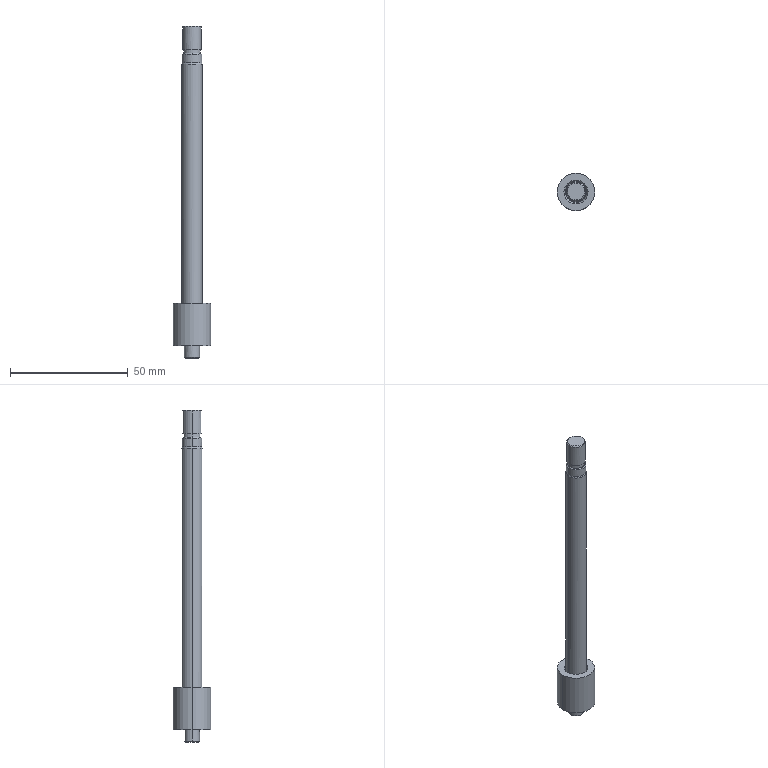Part | SolidWorks | features BaseBody 2, CombineBodies 1, Scale 1 | 1 solid | 50 faces | box 15.92 x 15.92 x 140.8 mm | volume 10674 mm3 | cylinder 22 | cone 17 | plane 11 | commonest cylinder face diameters 8.8 x6 4.8 x2 5.6 x2 6.4 x2 7.04 x2 7.2 x2
STEP:
#1=CARTESIAN_POINT('',(0.,-3.6,68.963));
#2=VERTEX_POINT('',#1);
#3=CARTESIAN_POINT('',(3.6,0.,68.963));
#4=VERTEX_POINT('',#3);
#5=CARTESIAN_POINT('',(0.,0.,68.963));
#6=DIRECTION('',(0.,0.,1.));
#7=DIRECTION('',(-1.,0.,0.));
#8=AXIS2_PLACEMENT_3D('',#5,#6,#7);
#9=CIRCLE('',#8,3.6);
#10=EDGE_CURVE('',#2,#4,#9,.T.);
#11=ORIENTED_EDGE('',*,*,#10,.F.);
#12=CARTESIAN_POINT('',(0.,-4.,68.563));
#13=VERTEX_POINT('',#12);
#14=CARTESIAN_POINT('',(0.,-3.8,68.763));
#15=DIRECTION('',(0.,-0.7071,-0.7071));
#16=VECTOR('',#15,1000.);
#17=LINE('',#14,#16);
#18=EDGE_CURVE('',#2,#13,#17,.T.);
#19=ORIENTED_EDGE('',*,*,#18,.T.);
#20=CARTESIAN_POINT('',(4.,0.,68.563));
#21=VERTEX_POINT('',#20);
#22=CARTESIAN_POINT('',(0.,0.,68.563));
#23=DIRECTION('',(0.,0.,1.));
#24=DIRECTION('',(-1.,0.,0.));
#25=AXIS2_PLACEMENT_3D('',#22,#23,#24);
#26=CIRCLE('',#25,4.);
#27=EDGE_CURVE('',#13,#21,#26,.T.);
#28=ORIENTED_EDGE('',*,*,#27,.T.);
#29=CARTESIAN_POINT('',(3.6,0.000000096,68.963));
#30=DIRECTION('',(0.7071,-0.000000028,-0.7071));
#31=VECTOR('',#30,1000.);
#32=LINE('',#29,#31);
#33=EDGE_CURVE('',#4,#21,#32,.T.);
#34=ORIENTED_EDGE('',*,*,#33,.F.);
#35=EDGE_LOOP('',(#11,#19,#28,#34));
#36=FACE_OUTER_BOUND('',#35,.T.);
#37=CARTESIAN_POINT('',(0.,0.,68.763));
#38=DIRECTION('',(0.,0.,-1.));
#39=DIRECTION('',(0.,-1.,0.));
#40=AXIS2_PLACEMENT_3D('',#37,#38,#39);
#41=CONICAL_SURFACE('',#40,3.8,0.7854);
#42=ADVANCED_FACE('',(#36),#41,.T.);
#43=CARTESIAN_POINT('',(0.,-3.8,57.363));
#44=VERTEX_POINT('',#43);
#45=CARTESIAN_POINT('',(3.8,0.,57.363));
#46=VERTEX_POINT('',#45);
#47=CARTESIAN_POINT('',(0.,0.,57.363));
#48=DIRECTION('',(0.,0.,1.));
#49=DIRECTION('',(-1.,0.,0.));
#50=AXIS2_PLACEMENT_3D('',#47,#48,#49);
#51=CIRCLE('',#50,3.8);
#52=EDGE_CURVE('',#44,#46,#51,.T.);
#53=ORIENTED_EDGE('',*,*,#52,.F.);
#54=CARTESIAN_POINT('',(0.,-4.2,56.963));
#55=VERTEX_POINT('',#54);
#56=CARTESIAN_POINT('',(0.,-4.,57.163));
#57=DIRECTION('',(0.,-0.7071,-0.7071));
#58=VECTOR('',#57,1000.);
#59=LINE('',#56,#58);
#60=EDGE_CURVE('',#44,#55,#59,.T.);
#61=ORIENTED_EDGE('',*,*,#60,.T.);
#62=CARTESIAN_POINT('',(4.2,0.,56.963));
#63=VERTEX_POINT('',#62);
#64=CARTESIAN_POINT('',(0.,0.,56.963));
#65=DIRECTION('',(0.,0.,1.));
#66=DIRECTION('',(-1.,0.,0.));
#67=AXIS2_PLACEMENT_3D('',#64,#65,#66);
#68=CIRCLE('',#67,4.2);
#69=EDGE_CURVE('',#55,#63,#68,.T.);
#70=ORIENTED_EDGE('',*,*,#69,.T.);
#71=CARTESIAN_POINT('',(3.8,0.000000099,57.363));
#72=DIRECTION('',(0.7071,-0.00000003,-0.7071));
#73=VECTOR('',#72,1000.);
#74=LINE('',#71,#73);
#75=EDGE_CURVE('',#46,#63,#74,.T.);
#76=ORIENTED_EDGE('',*,*,#75,.F.);
#77=EDGE_LOOP('',(#53,#61,#70,#76));
#78=FACE_OUTER_BOUND('',#77,.T.);
#79=CARTESIAN_POINT('',(0.,0.,57.163));
#80=DIRECTION('',(0.,0.,-1.));
#81=DIRECTION('',(0.,-1.,0.));
#82=AXIS2_PLACEMENT_3D('',#79,#80,#81);
#83=CONICAL_SURFACE('',#82,4.,0.7854);
#84=ADVANCED_FACE('',(#78),#83,.T.);
#85=CARTESIAN_POINT('',(-2.8,0.,-71.837));
#86=VERTEX_POINT('',#85);
#87=CARTESIAN_POINT('',(0.,-2.8,-71.837));
#88=VERTEX_POINT('',#87);
#89=CARTESIAN_POINT('',(0.,0.,-71.837));
#90=DIRECTION('',(0.,0.,1.));
#91=DIRECTION('',(-1.,0.,0.));
#92=AXIS2_PLACEMENT_3D('',#89,#90,#91);
#93=CIRCLE('',#92,2.8);
#94=EDGE_CURVE('',#86,#88,#93,.T.);
#95=ORIENTED_EDGE('',*,*,#94,.T.);
#96=CARTESIAN_POINT('',(0.,-3.2,-71.437));
#97=VERTEX_POINT('',#96);
#98=CARTESIAN_POINT('',(0.,-3.,-71.637));
#99=DIRECTION('',(0.,-0.7071,0.7071));
#100=VECTOR('',#99,1000.);
#101=LINE('',#98,#100);
#102=EDGE_CURVE('',#88,#97,#101,.T.);
#103=ORIENTED_EDGE('',*,*,#102,.T.);
#104=CARTESIAN_POINT('',(-3.2,0.,-71.437));
#105=VERTEX_POINT('',#104);
#106=CARTESIAN_POINT('',(0.,0.,-71.437));
#107=DIRECTION('',(0.,0.,1.));
#108=DIRECTION('',(-1.,0.,0.));
#109=AXIS2_PLACEMENT_3D('',#106,#107,#108);
#110=CIRCLE('',#109,3.2);
#111=EDGE_CURVE('',#105,#97,#110,.T.);
#112=ORIENTED_EDGE('',*,*,#111,.F.);
#113=CARTESIAN_POINT('',(-3.2,0.000000012,-71.437));
#114=DIRECTION('',(0.7071,0.000000004,-0.7071));
#115=VECTOR('',#114,1000.);
#116=LINE('',#113,#115);
#117=EDGE_CURVE('',#105,#86,#116,.T.);
#118=ORIENTED_EDGE('',*,*,#117,.T.);
#119=EDGE_LOOP('',(#95,#103,#112,#118));
#120=FACE_OUTER_BOUND('',#119,.T.);
#121=CARTESIAN_POINT('',(0.,0.,-71.637));
#122=DIRECTION('',(0.,0.,1.));
#123=DIRECTION('',(0.,-1.,0.));
#124=AXIS2_PLACEMENT_3D('',#121,#122,#123);
#125=CONICAL_SURFACE('',#124,3.,0.7854);
#126=ADVANCED_FACE('',(#120),#125,.T.);
#127=CARTESIAN_POINT('',(0.,-4.4,-49.837));
#128=VERTEX_POINT('',#127);
#129=CARTESIAN_POINT('',(4.4,0.,-49.837));
#130=VERTEX_POINT('',#129);
#131=CARTESIAN_POINT('',(0.,0.,-49.837));
#132=DIRECTION('',(0.,0.,1.));
#133=DIRECTION('',(-1.,0.,0.));
#134=AXIS2_PLACEMENT_3D('',#131,#132,#133);
#135=CIRCLE('',#134,4.4);
#136=EDGE_CURVE('',#128,#130,#135,.T.);
#137=ORIENTED_EDGE('',*,*,#136,.F.);
#138=CARTESIAN_POINT('',(0.,-5.093,-48.637));
#139=VERTEX_POINT('',#138);
#140=CARTESIAN_POINT('',(0.,-4.746,-49.237));
#141=DIRECTION('',(0.,-0.5,0.866));
#142=VECTOR('',#141,1000.);
#143=LINE('',#140,#142);
#144=EDGE_CURVE('',#128,#139,#143,.T.);
#145=ORIENTED_EDGE('',*,*,#144,.T.);
#146=CARTESIAN_POINT('',(5.093,0.,-48.637));
#147=VERTEX_POINT('',#146);
#148=CARTESIAN_POINT('',(0.,0.,-48.637));
#149=DIRECTION('',(0.,0.,1.));
#150=DIRECTION('',(-1.,0.,0.));
#151=AXIS2_PLACEMENT_3D('',#148,#149,#150);
#152=CIRCLE('',#151,5.093);
#153=EDGE_CURVE('',#139,#147,#152,.T.);
#154=ORIENTED_EDGE('',*,*,#153,.T.);
#155=CARTESIAN_POINT('',(4.4,0.000000001,-49.837));
#156=DIRECTION('',(0.5,0.,0.866));
#157=VECTOR('',#156,1000.);
#158=LINE('',#155,#157);
#159=EDGE_CURVE('',#130,#147,#158,.T.);
#160=ORIENTED_EDGE('',*,*,#159,.F.);
#161=EDGE_LOOP('',(#137,#145,#154,#160));
#162=FACE_OUTER_BOUND('',#161,.T.);
#163=CARTESIAN_POINT('',(0.,0.,-49.237));
#164=DIRECTION('',(0.,0.,1.));
#165=DIRECTION('',(0.,-1.,0.));
#166=AXIS2_PLACEMENT_3D('',#163,#164,#165);
#167=CONICAL_SURFACE('',#166,4.746,0.5236);
#168=ADVANCED_FACE('',(#162),#167,.F.);
#169=CARTESIAN_POINT('',(-7.96,0.,-48.637));
#170=VERTEX_POINT('',#169);
#171=CARTESIAN_POINT('',(7.96,0.,-48.637));
#172=VERTEX_POINT('',#171);
#173=CARTESIAN_POINT('',(0.,0.,-48.637));
#174=DIRECTION('',(0.,0.,-1.));
#175=DIRECTION('',(-1.,0.,0.));
#176=AXIS2_PLACEMENT_3D('',#173,#174,#175);
#177=CIRCLE('',#176,7.96);
#178=EDGE_CURVE('',#170,#172,#177,.T.);
#179=ORIENTED_EDGE('',*,*,#178,.F.);
#180=CARTESIAN_POINT('',(0.,0.,-48.637));
#181=DIRECTION('',(0.,0.,1.));
#182=DIRECTION('',(-1.,0.,0.));
#183=AXIS2_PLACEMENT_3D('',#180,#181,#182);
#184=CIRCLE('',#183,7.96);
#185=EDGE_CURVE('',#170,#172,#184,.T.);
#186=ORIENTED_EDGE('',*,*,#185,.T.);
#187=EDGE_LOOP('',(#179,#186));
#188=FACE_OUTER_BOUND('',#187,.T.);
#189=CARTESIAN_POINT('',(-5.093,0.,-48.637));
#190=VERTEX_POINT('',#189);
#191=CARTESIAN_POINT('',(0.,0.,-48.637));
#192=DIRECTION('',(0.,0.,1.));
#193=DIRECTION('',(1.,0.,0.));
#194=AXIS2_PLACEMENT_3D('',#191,#192,#193);
#195=CIRCLE('',#194,5.093);
#196=EDGE_CURVE('',#147,#190,#195,.T.);
#197=ORIENTED_EDGE('',*,*,#196,.F.);
#198=ORIENTED_EDGE('',*,*,#153,.F.);
#199=CARTESIAN_POINT('',(0.,0.,-48.637));
#200=DIRECTION('',(0.,0.,1.));
#201=DIRECTION('',(-1.,0.,0.));
#202=AXIS2_PLACEMENT_3D('',#199,#200,#201);
#203=CIRCLE('',#202,5.093);
#204=EDGE_CURVE('',#190,#139,#203,.T.);
#205=ORIENTED_EDGE('',*,*,#204,.F.);
#206=EDGE_LOOP('',(#197,#198,#205));
#207=FACE_BOUND('',#206,.T.);
#208=CARTESIAN_POINT('',(0.,0.,-48.637));
#209=DIRECTION('',(0.,0.,-1.));
#210=DIRECTION('',(0.,-1.,0.));
#211=AXIS2_PLACEMENT_3D('',#208,#209,#210);
#212=PLANE('',#211);
#213=ADVANCED_FACE('',(#188,#207),#212,.F.);
#214=CARTESIAN_POINT('',(-7.96,0.,-66.637));
#215=VERTEX_POINT('',#214);
#216=CARTESIAN_POINT('',(7.96,0.,-66.637));
#217=VERTEX_POINT('',#216);
#218=CARTESIAN_POINT('',(0.,0.,-66.637));
#219=DIRECTION('',(0.,0.,1.));
#220=DIRECTION('',(-1.,0.,0.));
#221=AXIS2_PLACEMENT_3D('',#218,#219,#220);
#222=CIRCLE('',#221,7.96);
#223=EDGE_CURVE('',#215,#217,#222,.T.);
#224=ORIENTED_EDGE('',*,*,#223,.T.);
#225=CARTESIAN_POINT('',(7.96,0.,-66.637));
#226=DIRECTION('',(0.,0.,1.));
#227=VECTOR('',#226,1000.);
#228=LINE('',#225,#227);
#229=EDGE_CURVE('',#217,#172,#228,.T.);
#230=ORIENTED_EDGE('',*,*,#229,.T.);
#231=ORIENTED_EDGE('',*,*,#185,.F.);
#232=CARTESIAN_POINT('',(-7.96,0.,-66.637));
#233=DIRECTION('',(0.,0.,1.));
#234=VECTOR('',#233,1000.);
#235=LINE('',#232,#234);
#236=EDGE_CURVE('',#215,#170,#235,.T.);
#237=ORIENTED_EDGE('',*,*,#236,.F.);
#238=EDGE_LOOP('',(#224,#230,#231,#237));
#239=FACE_OUTER_BOUND('',#238,.T.);
#240=CARTESIAN_POINT('',(0.,0.,-47.737));
#241=DIRECTION('',(0.,0.,-1.));
#242=DIRECTION('',(1.,0.,0.));
#243=AXIS2_PLACEMENT_3D('',#240,#241,#242);
#244=CYLINDRICAL_SURFACE('',#243,7.96);
#245=ADVANCED_FACE('',(#239),#244,.T.);
#246=ORIENTED_EDGE('',*,*,#178,.T.);
#247=ORIENTED_EDGE('',*,*,#229,.F.);
#248=CARTESIAN_POINT('',(0.,0.,-66.637));
#249=DIRECTION('',(0.,0.,-1.));
#250=DIRECTION('',(-1.,0.,0.));
#251=AXIS2_PLACEMENT_3D('',#248,#249,#250);
#252=CIRCLE('',#251,7.96);
#253=EDGE_CURVE('',#215,#217,#252,.T.);
#254=ORIENTED_EDGE('',*,*,#253,.F.);
#255=ORIENTED_EDGE('',*,*,#236,.T.);
#256=EDGE_LOOP('',(#246,#247,#254,#255));
#257=FACE_OUTER_BOUND('',#256,.T.);
#258=CARTESIAN_POINT('',(0.,0.,-47.737));
#259=DIRECTION('',(0.,0.,-1.));
#260=DIRECTION('',(1.,0.,0.));
#261=AXIS2_PLACEMENT_3D('',#258,#259,#260);
#262=CYLINDRICAL_SURFACE('',#261,7.96);
#263=ADVANCED_FACE('',(#257),#262,.T.);
#264=CARTESIAN_POINT('',(3.2,-0.000000008,-66.637));
#265=VERTEX_POINT('',#264);
#266=CARTESIAN_POINT('',(-3.2,0.,-66.637));
#267=VERTEX_POINT('',#266);
#268=CARTESIAN_POINT('',(0.,0.,-66.637));
#269=DIRECTION('',(0.,0.,-1.));
#270=DIRECTION('',(-1.,0.,0.));
#271=AXIS2_PLACEMENT_3D('',#268,#269,#270);
#272=CIRCLE('',#271,3.2);
#273=EDGE_CURVE('',#265,#267,#272,.T.);
#274=ORIENTED_EDGE('',*,*,#273,.F.);
#275=CARTESIAN_POINT('',(0.,0.,-66.637));
#276=DIRECTION('',(0.,0.,-1.));
#277=DIRECTION('',(-1.,0.,0.));
#278=AXIS2_PLACEMENT_3D('',#275,#276,#277);
#279=CIRCLE('',#278,3.2);
#280=EDGE_CURVE('',#267,#265,#279,.T.);
#281=ORIENTED_EDGE('',*,*,#280,.F.);
#282=EDGE_LOOP('',(#274,#281));
#283=FACE_BOUND('',#282,.T.);
#284=ORIENTED_EDGE('',*,*,#223,.F.);
#285=ORIENTED_EDGE('',*,*,#253,.T.);
#286=EDGE_LOOP('',(#284,#285));
#287=FACE_OUTER_BOUND('',#286,.T.);
#288=CARTESIAN_POINT('',(0.,0.,-66.637));
#289=DIRECTION('',(0.,0.,-1.));
#290=DIRECTION('',(0.,-1.,0.));
#291=AXIS2_PLACEMENT_3D('',#288,#289,#290);
#292=PLANE('',#291);
#293=ADVANCED_FACE('',(#283,#287),#292,.T.);
#294=ORIENTED_EDGE('',*,*,#144,.F.);
#295=CARTESIAN_POINT('',(-4.4,0.,-49.837));
#296=VERTEX_POINT('',#295);
#297=CARTESIAN_POINT('',(0.,0.,-49.837));
#298=DIRECTION('',(0.,0.,1.));
#299=DIRECTION('',(-1.,0.,0.));
#300=AXIS2_PLACEMENT_3D('',#297,#298,#299);
#301=CIRCLE('',#300,4.4);
#302=EDGE_CURVE('',#296,#128,#301,.T.);
#303=ORIENTED_EDGE('',*,*,#302,.F.);
#304=CARTESIAN_POINT('',(-4.4,-0.000000001,-49.837));
#305=DIRECTION('',(-0.5,0.,0.866));
#306=VECTOR('',#305,1000.);
#307=LINE('',#304,#306);
#308=EDGE_CURVE('',#296,#190,#307,.T.);
#309=ORIENTED_EDGE('',*,*,#308,.T.);
#310=ORIENTED_EDGE('',*,*,#204,.T.);
#311=EDGE_LOOP('',(#294,#303,#309,#310));
#312=FACE_OUTER_BOUND('',#311,.T.);
#313=CARTESIAN_POINT('',(0.,0.,-49.237));
#314=DIRECTION('',(0.,0.,1.));
#315=DIRECTION('',(0.,-1.,0.));
#316=AXIS2_PLACEMENT_3D('',#313,#314,#315);
#317=CONICAL_SURFACE('',#316,4.746,0.5236);
#318=ADVANCED_FACE('',(#312),#317,.F.);
#319=ORIENTED_EDGE('',*,*,#159,.T.);
#320=ORIENTED_EDGE('',*,*,#196,.T.);
#321=ORIENTED_EDGE('',*,*,#308,.F.);
#322=CARTESIAN_POINT('',(0.,0.,-49.837));
#323=DIRECTION('',(0.,0.,1.));
#324=DIRECTION('',(1.,0.,0.));
#325=AXIS2_PLACEMENT_3D('',#322,#323,#324);
#326=CIRCLE('',#325,4.4);
#327=EDGE_CURVE('',#130,#296,#326,.T.);
#328=ORIENTED_EDGE('',*,*,#327,.F.);
#329=EDGE_LOOP('',(#319,#320,#321,#328));
#330=FACE_OUTER_BOUND('',#329,.T.);
#331=CARTESIAN_POINT('',(0.,0.,-49.237));
#332=DIRECTION('',(0.,0.,1.));
#333=DIRECTION('',(0.,-1.,0.));
#334=AXIS2_PLACEMENT_3D('',#331,#332,#333);
#335=CONICAL_SURFACE('',#334,4.746,0.5236);
#336=ADVANCED_FACE('',(#330),#335,.F.);
#337=CARTESIAN_POINT('',(2.8,0.,-71.837));
#338=VERTEX_POINT('',#337);
#339=CARTESIAN_POINT('',(0.,0.,-71.837));
#340=DIRECTION('',(0.,0.,1.));
#341=DIRECTION('',(1.,0.,0.));
#342=AXIS2_PLACEMENT_3D('',#339,#340,#341);
#343=CIRCLE('',#342,2.8);
#344=EDGE_CURVE('',#338,#86,#343,.T.);
#345=ORIENTED_EDGE('',*,*,#344,.F.);
#346=CARTESIAN_POINT('',(0.,0.,-71.837));
#347=DIRECTION('',(0.,0.,1.));
#348=DIRECTION('',(-1.,0.,0.));
#349=AXIS2_PLACEMENT_3D('',#346,#347,#348);
#350=CIRCLE('',#349,2.8);
#351=EDGE_CURVE('',#88,#338,#350,.T.);
#352=ORIENTED_EDGE('',*,*,#351,.F.);
#353=ORIENTED_EDGE('',*,*,#94,.F.);
#354=EDGE_LOOP('',(#345,#352,#353));
#355=FACE_OUTER_BOUND('',#354,.T.);
#356=CARTESIAN_POINT('',(0.,0.,-71.837));
#357=DIRECTION('',(0.,0.,-1.));
#358=DIRECTION('',(0.,-1.,0.));
#359=AXIS2_PLACEMENT_3D('',#356,#357,#358);
#360=PLANE('',#359);
#361=ADVANCED_FACE('',(#355),#360,.T.);
#362=ORIENTED_EDGE('',*,*,#102,.F.);
#363=ORIENTED_EDGE('',*,*,#351,.T.);
#364=CARTESIAN_POINT('',(3.2,0.,-71.437));
#365=VERTEX_POINT('',#364);
#366=CARTESIAN_POINT('',(3.2,-0.000000012,-71.437));
#367=DIRECTION('',(-0.7071,-0.000000004,-0.7071));
#368=VECTOR('',#367,1000.);
#369=LINE('',#366,#368);
#370=EDGE_CURVE('',#365,#338,#369,.T.);
#371=ORIENTED_EDGE('',*,*,#370,.F.);
#372=CARTESIAN_POINT('',(0.,0.,-71.437));
#373=DIRECTION('',(0.,0.,1.));
#374=DIRECTION('',(-1.,0.,0.));
#375=AXIS2_PLACEMENT_3D('',#372,#373,#374);
#376=CIRCLE('',#375,3.2);
#377=EDGE_CURVE('',#97,#365,#376,.T.);
#378=ORIENTED_EDGE('',*,*,#377,.F.);
#379=EDGE_LOOP('',(#362,#363,#371,#378));
#380=FACE_OUTER_BOUND('',#379,.T.);
#381=CARTESIAN_POINT('',(0.,0.,-71.637));
#382=DIRECTION('',(0.,0.,1.));
#383=DIRECTION('',(0.,-1.,0.));
#384=AXIS2_PLACEMENT_3D('',#381,#382,#383);
#385=CONICAL_SURFACE('',#384,3.,0.7854);
#386=ADVANCED_FACE('',(#380),#385,.T.);
#387=ORIENTED_EDGE('',*,*,#370,.T.);
#388=ORIENTED_EDGE('',*,*,#344,.T.);
#389=ORIENTED_EDGE('',*,*,#117,.F.);
#390=CARTESIAN_POINT('',(0.,0.,-71.437));
#391=DIRECTION('',(0.,0.,1.));
#392=DIRECTION('',(1.,0.,0.));
#393=AXIS2_PLACEMENT_3D('',#390,#391,#392);
#394=CIRCLE('',#393,3.2);
#395=EDGE_CURVE('',#365,#105,#394,.T.);
#396=ORIENTED_EDGE('',*,*,#395,.F.);
#397=EDGE_LOOP('',(#387,#388,#389,#396));
#398=FACE_OUTER_BOUND('',#397,.T.);
#399=CARTESIAN_POINT('',(0.,0.,-71.637));
#400=DIRECTION('',(0.,0.,1.));
#401=DIRECTION('',(0.,-1.,0.));
#402=AXIS2_PLACEMENT_3D('',#399,#400,#401);
#403=CONICAL_SURFACE('',#402,3.,0.7854);
#404=ADVANCED_FACE('',(#398),#403,.T.);
#405=CARTESIAN_POINT('',(-3.2,0.000000012,-71.437));
#406=DIRECTION('',(-0.000000001,-0.000000001,1.));
#407=VECTOR('',#406,1000.);
#408=LINE('',#405,#407);
#409=EDGE_CURVE('',#105,#267,#408,.T.);
#410=ORIENTED_EDGE('',*,*,#409,.T.);
#411=ORIENTED_EDGE('',*,*,#280,.T.);
#412=CARTESIAN_POINT('',(3.2,-0.000000012,-71.437));
#413=DIRECTION('',(0.000000001,0.000000001,1.));
#414=VECTOR('',#413,1000.);
#415=LINE('',#412,#414);
#416=EDGE_CURVE('',#365,#265,#415,.T.);
#417=ORIENTED_EDGE('',*,*,#416,.F.);
#418=ORIENTED_EDGE('',*,*,#395,.T.);
#419=EDGE_LOOP('',(#410,#411,#417,#418));
#420=FACE_OUTER_BOUND('',#419,.T.);
#421=CARTESIAN_POINT('',(0.,0.,76.239));
#422=DIRECTION('',(0.,0.,-1.));
#423=DIRECTION('',(1.,0.,0.));
#424=AXIS2_PLACEMENT_3D('',#421,#422,#423);
#425=CYLINDRICAL_SURFACE('',#424,3.2);
#426=ADVANCED_FACE('',(#420),#425,.T.);
#427=ORIENTED_EDGE('',*,*,#416,.T.);
#428=ORIENTED_EDGE('',*,*,#273,.T.);
#429=ORIENTED_EDGE('',*,*,#409,.F.);
#430=ORIENTED_EDGE('',*,*,#111,.T.);
#431=ORIENTED_EDGE('',*,*,#377,.T.);
#432=EDGE_LOOP('',(#427,#428,#429,#430,#431));
#433=FACE_OUTER_BOUND('',#432,.T.);
#434=CARTESIAN_POINT('',(0.,0.,76.239));
#435=DIRECTION('',(0.,0.,-1.));
#436=DIRECTION('',(1.,0.,0.));
#437=AXIS2_PLACEMENT_3D('',#434,#435,#436);
#438=CYLINDRICAL_SURFACE('',#437,3.2);
#439=ADVANCED_FACE('',(#433),#438,.T.);
#440=CARTESIAN_POINT('',(-4.4,0.,52.813));
#441=VERTEX_POINT('',#440);
#442=CARTESIAN_POINT('',(-4.4,0.,-51.197));
#443=DIRECTION('',(0.,0.,1.));
#444=VECTOR('',#443,1000.);
#445=LINE('',#442,#444);
#446=EDGE_CURVE('',#296,#441,#445,.T.);
#447=ORIENTED_EDGE('',*,*,#446,.F.);
#448=ORIENTED_EDGE('',*,*,#302,.T.);
#449=ORIENTED_EDGE('',*,*,#136,.T.);
#450=CARTESIAN_POINT('',(4.4,0.,52.813));
#451=VERTEX_POINT('',#450);
#452=CARTESIAN_POINT('',(4.4,0.,-51.197));
#453=DIRECTION('',(0.,0.,1.));
#454=VECTOR('',#453,1000.);
#455=LINE('',#452,#454);
#456=EDGE_CURVE('',#130,#451,#455,.T.);
#457=ORIENTED_EDGE('',*,*,#456,.T.);
#458=CARTESIAN_POINT('',(0.,0.,52.813));
#459=DIRECTION('',(0.,0.,1.));
#460=DIRECTION('',(-1.,0.,0.));
#461=AXIS2_PLACEMENT_3D('',#458,#459,#460);
#462=CIRCLE('',#461,4.4);
#463=EDGE_CURVE('',#441,#451,#462,.T.);
#464=ORIENTED_EDGE('',*,*,#463,.F.);
#465=EDGE_LOOP('',(#447,#448,#449,#457,#464));
#466=FACE_OUTER_BOUND('',#465,.T.);
#467=CARTESIAN_POINT('',(0.,0.,76.239));
#468=DIRECTION('',(0.,0.,-1.));
#469=DIRECTION('',(1.,0.,0.));
#470=AXIS2_PLACEMENT_3D('',#467,#468,#469);
#471=CYLINDRICAL_SURFACE('',#470,4.4);
#472=ADVANCED_FACE('',(#466),#471,.T.);
#473=ORIENTED_EDGE('',*,*,#456,.F.);
#474=ORIENTED_EDGE('',*,*,#327,.T.);
#475=ORIENTED_EDGE('',*,*,#446,.T.);
#476=CARTESIAN_POINT('',(0.,0.,52.813));
#477=DIRECTION('',(0.,0.,-1.));
#478=DIRECTION('',(-1.,0.,0.));
#479=AXIS2_PLACEMENT_3D('',#476,#477,#478);
#480=CIRCLE('',#479,4.4);
#481=EDGE_CURVE('',#441,#451,#480,.T.);
#482=ORIENTED_EDGE('',*,*,#481,.T.);
#483=EDGE_LOOP('',(#473,#474,#475,#482));
#484=FACE_OUTER_BOUND('',#483,.T.);
#485=CARTESIAN_POINT('',(0.,0.,76.239));
#486=DIRECTION('',(0.,0.,-1.));
#487=DIRECTION('',(1.,0.,0.));
#488=AXIS2_PLACEMENT_3D('',#485,#486,#487);
#489=CYLINDRICAL_SURFACE('',#488,4.4);
#490=ADVANCED_FACE('',(#484),#489,.T.);
#491=CARTESIAN_POINT('',(-4.2,0.,53.363));
#492=VERTEX_POINT('',#491);
#493=CARTESIAN_POINT('',(4.2,0.,53.363));
#494=VERTEX_POINT('',#493);
#495=CARTESIAN_POINT('',(0.,0.,53.363));
#496=DIRECTION('',(0.,0.,-1.));
#497=DIRECTION('',(-1.,0.,0.));
#498=AXIS2_PLACEMENT_3D('',#495,#496,#497);
#499=CIRCLE('',#498,4.2);
#500=EDGE_CURVE('',#492,#494,#499,.T.);
#501=ORIENTED_EDGE('',*,*,#500,.T.);
#502=CARTESIAN_POINT('',(4.4,0.,52.813));
#503=DIRECTION('',(-0.342,0.,0.9397));
#504=VECTOR('',#503,1000.);
#505=LINE('',#502,#504);
#506=EDGE_CURVE('',#451,#494,#505,.T.);
#507=ORIENTED_EDGE('',*,*,#506,.F.);
#508=ORIENTED_EDGE('',*,*,#481,.F.);
#509=CARTESIAN_POINT('',(-4.4,0.,52.813));
#510=DIRECTION('',(0.342,0.,0.9397));
#511=VECTOR('',#510,1000.);
#512=LINE('',#509,#511);
#513=EDGE_CURVE('',#441,#492,#512,.T.);
#514=ORIENTED_EDGE('',*,*,#513,.T.);
#515=EDGE_LOOP('',(#501,#507,#508,#514));
#516=FACE_OUTER_BOUND('',#515,.T.);
#517=CARTESIAN_POINT('',(0.,0.,53.088));
#518=DIRECTION('',(0.,0.,-1.));
#519=DIRECTION('',(1.,0.,0.));
#520=AXIS2_PLACEMENT_3D('',#517,#518,#519);
#521=CONICAL_SURFACE('',#520,4.3,0.3491);
#522=ADVANCED_FACE('',(#516),#521,.T.);
#523=ORIENTED_EDGE('',*,*,#463,.T.);
#524=ORIENTED_EDGE('',*,*,#506,.T.);
#525=CARTESIAN_POINT('',(0.,0.,53.363));
#526=DIRECTION('',(0.,0.,1.));
#527=DIRECTION('',(-1.,0.,0.));
#528=AXIS2_PLACEMENT_3D('',#525,#526,#527);
#529=CIRCLE('',#528,4.2);
#530=EDGE_CURVE('',#492,#494,#529,.T.);
#531=ORIENTED_EDGE('',*,*,#530,.F.);
#532=ORIENTED_EDGE('',*,*,#513,.F.);
#533=EDGE_LOOP('',(#523,#524,#531,#532));
#534=FACE_OUTER_BOUND('',#533,.T.);
#535=CARTESIAN_POINT('',(0.,0.,53.088));
#536=DIRECTION('',(0.,0.,-1.));
#537=DIRECTION('',(1.,0.,0.));
#538=AXIS2_PLACEMENT_3D('',#535,#536,#537);
#539=CONICAL_SURFACE('',#538,4.3,0.3491);
#540=ADVANCED_FACE('',(#534),#539,.T.);
#541=CARTESIAN_POINT('',(-4.2,0.,56.963));
#542=VERTEX_POINT('',#541);
#543=CARTESIAN_POINT('',(-4.2,0.,53.363));
#544=DIRECTION('',(0.000000004,-0.000000023,1.));
#545=VECTOR('',#544,1000.);
#546=LINE('',#543,#545);
#547=EDGE_CURVE('',#492,#542,#546,.T.);
#548=ORIENTED_EDGE('',*,*,#547,.F.);
#549=ORIENTED_EDGE('',*,*,#530,.T.);
#550=CARTESIAN_POINT('',(4.2,0.,53.363));
#551=DIRECTION('',(-0.000000004,0.000000023,1.));
#552=VECTOR('',#551,1000.);
#553=LINE('',#550,#552);
#554=EDGE_CURVE('',#494,#63,#553,.T.);
#555=ORIENTED_EDGE('',*,*,#554,.T.);
#556=ORIENTED_EDGE('',*,*,#69,.F.);
#557=CARTESIAN_POINT('',(0.,0.,56.963));
#558=DIRECTION('',(0.,0.,1.));
#559=DIRECTION('',(-1.,0.,0.));
#560=AXIS2_PLACEMENT_3D('',#557,#558,#559);
#561=CIRCLE('',#560,4.2);
#562=EDGE_CURVE('',#542,#55,#561,.T.);
#563=ORIENTED_EDGE('',*,*,#562,.F.);
#564=EDGE_LOOP('',(#548,#549,#555,#556,#563));
#565=FACE_OUTER_BOUND('',#564,.T.);
#566=CARTESIAN_POINT('',(0.,0.,76.239));
#567=DIRECTION('',(0.,0.,-1.));
#568=DIRECTION('',(1.,0.,0.));
#569=AXIS2_PLACEMENT_3D('',#566,#567,#568);
#570=CYLINDRICAL_SURFACE('',#569,4.2);
#571=ADVANCED_FACE('',(#565),#570,.T.);
#572=ORIENTED_EDGE('',*,*,#60,.F.);
#573=CARTESIAN_POINT('',(-3.8,0.,57.363));
#574=VERTEX_POINT('',#573);
#575=CARTESIAN_POINT('',(0.,0.,57.363));
#576=DIRECTION('',(0.,0.,1.));
#577=DIRECTION('',(-1.,0.,0.));
#578=AXIS2_PLACEMENT_3D('',#575,#576,#577);
#579=CIRCLE('',#578,3.8);
#580=EDGE_CURVE('',#574,#44,#579,.T.);
#581=ORIENTED_EDGE('',*,*,#580,.F.);
#582=CARTESIAN_POINT('',(-3.8,-0.000000099,57.363));
#583=DIRECTION('',(-0.7071,0.00000003,-0.7071));
#584=VECTOR('',#583,1000.);
#585=LINE('',#582,#584);
#586=EDGE_CURVE('',#574,#542,#585,.T.);
#587=ORIENTED_EDGE('',*,*,#586,.T.);
#588=ORIENTED_EDGE('',*,*,#562,.T.);
#589=EDGE_LOOP('',(#572,#581,#587,#588));
#590=FACE_OUTER_BOUND('',#589,.T.);
#591=CARTESIAN_POINT('',(0.,0.,57.163));
#592=DIRECTION('',(0.,0.,-1.));
#593=DIRECTION('',(0.,-1.,0.));
#594=AXIS2_PLACEMENT_3D('',#591,#592,#593);
#595=CONICAL_SURFACE('',#594,4.,0.7854);
#596=ADVANCED_FACE('',(#590),#595,.T.);
#597=CARTESIAN_POINT('',(0.,0.,57.363));
#598=DIRECTION('',(0.,0.,1.));
#599=DIRECTION('',(1.,0.,0.));
#600=AXIS2_PLACEMENT_3D('',#597,#598,#599);
#601=CIRCLE('',#600,3.8);
#602=EDGE_CURVE('',#46,#574,#601,.T.);
#603=ORIENTED_EDGE('',*,*,#602,.T.);
#604=ORIENTED_EDGE('',*,*,#580,.T.);
#605=ORIENTED_EDGE('',*,*,#52,.T.);
#606=EDGE_LOOP('',(#603,#604,#605));
#607=FACE_OUTER_BOUND('',#606,.T.);
#608=CARTESIAN_POINT('',(-3.6,0.,57.363));
#609=VERTEX_POINT('',#608);
#610=CARTESIAN_POINT('',(3.6,0.,57.363));
#611=VERTEX_POINT('',#610);
#612=CARTESIAN_POINT('',(0.,0.,57.363));
#613=DIRECTION('',(0.,0.,-1.));
#614=DIRECTION('',(-1.,0.,0.));
#615=AXIS2_PLACEMENT_3D('',#612,#613,#614);
#616=CIRCLE('',#615,3.6);
#617=EDGE_CURVE('',#609,#611,#616,.T.);
#618=ORIENTED_EDGE('',*,*,#617,.T.);
#619=CARTESIAN_POINT('',(0.,0.,57.363));
#620=DIRECTION('',(0.,0.,1.));
#621=DIRECTION('',(-1.,0.,0.));
#622=AXIS2_PLACEMENT_3D('',#619,#620,#621);
#623=CIRCLE('',#622,3.6);
#624=EDGE_CURVE('',#609,#611,#623,.T.);
#625=ORIENTED_EDGE('',*,*,#624,.F.);
#626=EDGE_LOOP('',(#618,#625));
#627=FACE_BOUND('',#626,.T.);
#628=CARTESIAN_POINT('',(0.,0.,57.363));
#629=DIRECTION('',(0.,0.,-1.));
#630=DIRECTION('',(0.,-1.,0.));
#631=AXIS2_PLACEMENT_3D('',#628,#629,#630);
#632=PLANE('',#631);
#633=ADVANCED_FACE('',(#607,#627),#632,.F.);
#634=ORIENTED_EDGE('',*,*,#624,.T.);
#635=CARTESIAN_POINT('',(3.6,0.,58.963));
#636=VERTEX_POINT('',#635);
#637=CARTESIAN_POINT('',(3.6,0.,57.363));
#638=DIRECTION('',(0.,0.,1.));
#639=VECTOR('',#638,1000.);
#640=LINE('',#637,#639);
#641=EDGE_CURVE('',#611,#636,#640,.T.);
#642=ORIENTED_EDGE('',*,*,#641,.T.);
#643=CARTESIAN_POINT('',(-3.6,0.,58.963));
#644=VERTEX_POINT('',#643);
#645=CARTESIAN_POINT('',(0.,0.,58.963));
#646=DIRECTION('',(0.,0.,1.));
#647=DIRECTION('',(-1.,0.,0.));
#648=AXIS2_PLACEMENT_3D('',#645,#646,#647);
#649=CIRCLE('',#648,3.6);
#650=EDGE_CURVE('',#644,#636,#649,.T.);
#651=ORIENTED_EDGE('',*,*,#650,.F.);
#652=CARTESIAN_POINT('',(-3.6,0.,57.363));
#653=DIRECTION('',(0.,0.,1.));
#654=VECTOR('',#653,1000.);
#655=LINE('',#652,#654);
#656=EDGE_CURVE('',#609,#644,#655,.T.);
#657=ORIENTED_EDGE('',*,*,#656,.F.);
#658=EDGE_LOOP('',(#634,#642,#651,#657));
#659=FACE_OUTER_BOUND('',#658,.T.);
#660=CARTESIAN_POINT('',(0.,0.,76.239));
#661=DIRECTION('',(0.,0.,-1.));
#662=DIRECTION('',(1.,0.,0.));
#663=AXIS2_PLACEMENT_3D('',#660,#661,#662);
#664=CYLINDRICAL_SURFACE('',#663,3.6);
#665=ADVANCED_FACE('',(#659),#664,.T.);
#666=CARTESIAN_POINT('',(0.,0.,58.963));
#667=DIRECTION('',(0.,0.,-1.));
#668=DIRECTION('',(-1.,0.,0.));
#669=AXIS2_PLACEMENT_3D('',#666,#667,#668);
#670=CIRCLE('',#669,3.6);
#671=EDGE_CURVE('',#644,#636,#670,.T.);
#672=ORIENTED_EDGE('',*,*,#671,.T.);
#673=ORIENTED_EDGE('',*,*,#641,.F.);
#674=ORIENTED_EDGE('',*,*,#617,.F.);
#675=ORIENTED_EDGE('',*,*,#656,.T.);
#676=EDGE_LOOP('',(#672,#673,#674,#675));
#677=FACE_OUTER_BOUND('',#676,.T.);
#678=CARTESIAN_POINT('',(0.,0.,76.239));
#679=DIRECTION('',(0.,0.,-1.));
#680=DIRECTION('',(1.,0.,0.));
#681=AXIS2_PLACEMENT_3D('',#678,#679,#680);
#682=CYLINDRICAL_SURFACE('',#681,3.6);
#683=ADVANCED_FACE('',(#677),#682,.T.);
#684=CARTESIAN_POINT('',(-4.,0.,58.963));
#685=VERTEX_POINT('',#684);
#686=CARTESIAN_POINT('',(4.,0.,58.963));
#687=VERTEX_POINT('',#686);
#688=CARTESIAN_POINT('',(0.,0.,58.963));
#689=DIRECTION('',(0.,0.,-1.));
#690=DIRECTION('',(-1.,0.,0.));
#691=AXIS2_PLACEMENT_3D('',#688,#689,#690);
#692=CIRCLE('',#691,4.);
#693=EDGE_CURVE('',#685,#687,#692,.T.);
#694=ORIENTED_EDGE('',*,*,#693,.T.);
#695=CARTESIAN_POINT('',(0.,0.,58.963));
#696=DIRECTION('',(0.,0.,1.));
#697=DIRECTION('',(-1.,0.,0.));
#698=AXIS2_PLACEMENT_3D('',#695,#696,#697);
#699=CIRCLE('',#698,4.);
#700=EDGE_CURVE('',#685,#687,#699,.T.);
#701=ORIENTED_EDGE('',*,*,#700,.F.);
#702=EDGE_LOOP('',(#694,#701));
#703=FACE_OUTER_BOUND('',#702,.T.);
#704=ORIENTED_EDGE('',*,*,#650,.T.);
#705=ORIENTED_EDGE('',*,*,#671,.F.);
#706=EDGE_LOOP('',(#704,#705));
#707=FACE_BOUND('',#706,.T.);
#708=CARTESIAN_POINT('',(0.,0.,58.963));
#709=DIRECTION('',(0.,0.,-1.));
#710=DIRECTION('',(0.,-1.,0.));
#711=AXIS2_PLACEMENT_3D('',#708,#709,#710);
#712=PLANE('',#711);
#713=ADVANCED_FACE('',(#703,#707),#712,.T.);
#714=CARTESIAN_POINT('',(-4.,0.,68.563));
#715=VERTEX_POINT('',#714);
#716=CARTESIAN_POINT('',(-4.,0.,58.963));
#717=DIRECTION('',(0.000000001,-0.000000008,1.));
#718=VECTOR('',#717,1000.);
#719=LINE('',#716,#718);
#720=EDGE_CURVE('',#685,#715,#719,.T.);
#721=ORIENTED_EDGE('',*,*,#720,.F.);
#722=ORIENTED_EDGE('',*,*,#700,.T.);
#723=CARTESIAN_POINT('',(4.,0.,58.963));
#724=DIRECTION('',(-0.000000001,0.000000008,1.));
#725=VECTOR('',#724,1000.);
#726=LINE('',#723,#725);
#727=EDGE_CURVE('',#687,#21,#726,.T.);
#728=ORIENTED_EDGE('',*,*,#727,.T.);
#729=ORIENTED_EDGE('',*,*,#27,.F.);
#730=CARTESIAN_POINT('',(0.,0.,68.563));
#731=DIRECTION('',(0.,0.,1.));
#732=DIRECTION('',(-1.,0.,0.));
#733=AXIS2_PLACEMENT_3D('',#730,#731,#732);
#734=CIRCLE('',#733,4.);
#735=EDGE_CURVE('',#715,#13,#734,.T.);
#736=ORIENTED_EDGE('',*,*,#735,.F.);
#737=EDGE_LOOP('',(#721,#722,#728,#729,#736));
#738=FACE_OUTER_BOUND('',#737,.T.);
#739=CARTESIAN_POINT('',(0.,0.,76.239));
#740=DIRECTION('',(0.,0.,-1.));
#741=DIRECTION('',(1.,0.,0.));
#742=AXIS2_PLACEMENT_3D('',#739,#740,#741);
#743=CYLINDRICAL_SURFACE('',#742,4.);
#744=ADVANCED_FACE('',(#738),#743,.T.);
#745=ORIENTED_EDGE('',*,*,#18,.F.);
#746=CARTESIAN_POINT('',(-3.6,0.,68.963));
#747=VERTEX_POINT('',#746);
#748=CARTESIAN_POINT('',(0.,0.,68.963));
#749=DIRECTION('',(0.,0.,1.));
#750=DIRECTION('',(-1.,0.,0.));
#751=AXIS2_PLACEMENT_3D('',#748,#749,#750);
#752=CIRCLE('',#751,3.6);
#753=EDGE_CURVE('',#747,#2,#752,.T.);
#754=ORIENTED_EDGE('',*,*,#753,.F.);
#755=CARTESIAN_POINT('',(-3.6,-0.000000096,68.963));
#756=DIRECTION('',(-0.7071,0.000000028,-0.7071));
#757=VECTOR('',#756,1000.);
#758=LINE('',#755,#757);
#759=EDGE_CURVE('',#747,#715,#758,.T.);
#760=ORIENTED_EDGE('',*,*,#759,.T.);
#761=ORIENTED_EDGE('',*,*,#735,.T.);
#762=EDGE_LOOP('',(#745,#754,#760,#761));
#763=FACE_OUTER_BOUND('',#762,.T.);
#764=CARTESIAN_POINT('',(0.,0.,68.763));
#765=DIRECTION('',(0.,0.,-1.));
#766=DIRECTION('',(0.,-1.,0.));
#767=AXIS2_PLACEMENT_3D('',#764,#765,#766);
#768=CONICAL_SURFACE('',#767,3.8,0.7854);
#769=ADVANCED_FACE('',(#763),#768,.T.);
#770=CARTESIAN_POINT('',(0.,0.,68.963));
#771=DIRECTION('',(0.,0.,1.));
#772=DIRECTION('',(1.,0.,0.));
#773=AXIS2_PLACEMENT_3D('',#770,#771,#772);
#774=CIRCLE('',#773,3.6);
#775=EDGE_CURVE('',#4,#747,#774,.T.);
#776=ORIENTED_EDGE('',*,*,#775,.T.);
#777=ORIENTED_EDGE('',*,*,#753,.T.);
#778=ORIENTED_EDGE('',*,*,#10,.T.);
#779=EDGE_LOOP('',(#776,#777,#778));
#780=FACE_OUTER_BOUND('',#779,.T.);
#781=CARTESIAN_POINT('',(0.,0.,68.963));
#782=DIRECTION('',(0.,0.,-1.));
#783=DIRECTION('',(0.,-1.,0.));
#784=AXIS2_PLACEMENT_3D('',#781,#782,#783);
#785=PLANE('',#784);
#786=ADVANCED_FACE('',(#780),#785,.F.);
#787=ORIENTED_EDGE('',*,*,#33,.T.);
#788=CARTESIAN_POINT('',(0.,0.,68.563));
#789=DIRECTION('',(0.,0.,1.));
#790=DIRECTION('',(1.,0.,0.));
#791=AXIS2_PLACEMENT_3D('',#788,#789,#790);
#792=CIRCLE('',#791,4.);
#793=EDGE_CURVE('',#21,#715,#792,.T.);
#794=ORIENTED_EDGE('',*,*,#793,.T.);
#795=ORIENTED_EDGE('',*,*,#759,.F.);
#796=ORIENTED_EDGE('',*,*,#775,.F.);
#797=EDGE_LOOP('',(#787,#794,#795,#796));
#798=FACE_OUTER_BOUND('',#797,.T.);
#799=CARTESIAN_POINT('',(0.,0.,68.763));
#800=DIRECTION('',(0.,0.,-1.));
#801=DIRECTION('',(0.,-1.,0.));
#802=AXIS2_PLACEMENT_3D('',#799,#800,#801);
#803=CONICAL_SURFACE('',#802,3.8,0.7854);
#804=ADVANCED_FACE('',(#798),#803,.T.);
#805=ORIENTED_EDGE('',*,*,#727,.F.);
#806=ORIENTED_EDGE('',*,*,#693,.F.);
#807=ORIENTED_EDGE('',*,*,#720,.T.);
#808=ORIENTED_EDGE('',*,*,#793,.F.);
#809=EDGE_LOOP('',(#805,#806,#807,#808));
#810=FACE_OUTER_BOUND('',#809,.T.);
#811=CARTESIAN_POINT('',(0.,0.,76.239));
#812=DIRECTION('',(0.,0.,-1.));
#813=DIRECTION('',(1.,0.,0.));
#814=AXIS2_PLACEMENT_3D('',#811,#812,#813);
#815=CYLINDRICAL_SURFACE('',#814,4.);
#816=ADVANCED_FACE('',(#810),#815,.T.);
#817=ORIENTED_EDGE('',*,*,#75,.T.);
#818=CARTESIAN_POINT('',(0.,0.,56.963));
#819=DIRECTION('',(0.,0.,1.));
#820=DIRECTION('',(1.,0.,0.));
#821=AXIS2_PLACEMENT_3D('',#818,#819,#820);
#822=CIRCLE('',#821,4.2);
#823=EDGE_CURVE('',#63,#542,#822,.T.);
#824=ORIENTED_EDGE('',*,*,#823,.T.);
#825=ORIENTED_EDGE('',*,*,#586,.F.);
#826=ORIENTED_EDGE('',*,*,#602,.F.);
#827=EDGE_LOOP('',(#817,#824,#825,#826));
#828=FACE_OUTER_BOUND('',#827,.T.);
#829=CARTESIAN_POINT('',(0.,0.,57.163));
#830=DIRECTION('',(0.,0.,-1.));
#831=DIRECTION('',(0.,-1.,0.));
#832=AXIS2_PLACEMENT_3D('',#829,#830,#831);
#833=CONICAL_SURFACE('',#832,4.,0.7854);
#834=ADVANCED_FACE('',(#828),#833,.T.);
#835=ORIENTED_EDGE('',*,*,#554,.F.);
#836=ORIENTED_EDGE('',*,*,#500,.F.);
#837=ORIENTED_EDGE('',*,*,#547,.T.);
#838=ORIENTED_EDGE('',*,*,#823,.F.);
#839=EDGE_LOOP('',(#835,#836,#837,#838));
#840=FACE_OUTER_BOUND('',#839,.T.);
#841=CARTESIAN_POINT('',(0.,0.,76.239));
#842=DIRECTION('',(0.,0.,-1.));
#843=DIRECTION('',(1.,0.,0.));
#844=AXIS2_PLACEMENT_3D('',#841,#842,#843);
#845=CYLINDRICAL_SURFACE('',#844,4.2);
#846=ADVANCED_FACE('',(#840),#845,.T.);
#847=CLOSED_SHELL('',(#42,#84,#126,#168,#213,#245,#263,#293,#318,#336,#361,#386,#404,#426,#439,#472,#490,#522,#540,#571,#596,#633,#665,#683,#713,#744,#769,#786,#804,#816,#834,#846));
#848=CARTESIAN_POINT('',(-3.52,0.,-51.197));
#849=VERTEX_POINT('',#848);
#850=CARTESIAN_POINT('',(3.52,0.,-51.197));
#851=VERTEX_POINT('',#850);
#852=CARTESIAN_POINT('',(0.,0.,-51.197));
#853=DIRECTION('',(0.,0.,-1.));
#854=DIRECTION('',(-1.,0.,0.));
#855=AXIS2_PLACEMENT_3D('',#852,#853,#854);
#856=CIRCLE('',#855,3.52);
#857=EDGE_CURVE('',#849,#851,#856,.T.);
#858=ORIENTED_EDGE('',*,*,#857,.T.);
#859=CARTESIAN_POINT('',(3.52,0.,-52.637));
#860=VERTEX_POINT('',#859);
#861=CARTESIAN_POINT('',(3.52,0.,-52.637));
#862=DIRECTION('',(0.,0.,1.));
#863=VECTOR('',#862,1000.);
#864=LINE('',#861,#863);
#865=EDGE_CURVE('',#860,#851,#864,.T.);
#866=ORIENTED_EDGE('',*,*,#865,.F.);
#867=CARTESIAN_POINT('',(-3.52,0.,-52.637));
#868=VERTEX_POINT('',#867);
#869=CARTESIAN_POINT('',(0.,0.,-52.637));
#870=DIRECTION('',(0.,0.,-1.));
#871=DIRECTION('',(-1.,0.,0.));
#872=AXIS2_PLACEMENT_3D('',#869,#870,#871);
#873=CIRCLE('',#872,3.52);
#874=EDGE_CURVE('',#868,#860,#873,.T.);
#875=ORIENTED_EDGE('',*,*,#874,.F.);
#876=CARTESIAN_POINT('',(-3.52,0.,-52.637));
#877=DIRECTION('',(0.,0.,1.));
#878=VECTOR('',#877,1000.);
#879=LINE('',#876,#878);
#880=EDGE_CURVE('',#868,#849,#879,.T.);
#881=ORIENTED_EDGE('',*,*,#880,.T.);
#882=EDGE_LOOP('',(#858,#866,#875,#881));
#883=FACE_OUTER_BOUND('',#882,.T.);
#884=CARTESIAN_POINT('',(0.,0.,76.239));
#885=DIRECTION('',(0.,0.,-1.));
#886=DIRECTION('',(1.,0.,0.));
#887=AXIS2_PLACEMENT_3D('',#884,#885,#886);
#888=CYLINDRICAL_SURFACE('',#887,3.52);
#889=ADVANCED_FACE('',(#883),#888,.T.);
#890=CARTESIAN_POINT('',(-4.4,0.,-52.637));
#891=VERTEX_POINT('',#890);
#892=CARTESIAN_POINT('',(4.4,0.,-52.637));
#893=VERTEX_POINT('',#892);
#894=CARTESIAN_POINT('',(0.,0.,-52.637));
#895=DIRECTION('',(0.,0.,1.));
#896=DIRECTION('',(-1.,0.,0.));
#897=AXIS2_PLACEMENT_3D('',#894,#895,#896);
#898=CIRCLE('',#897,4.4);
#899=EDGE_CURVE('',#891,#893,#898,.T.);
#900=ORIENTED_EDGE('',*,*,#899,.T.);
#901=CARTESIAN_POINT('',(0.,0.,-52.637));
#902=DIRECTION('',(0.,0.,-1.));
#903=DIRECTION('',(-1.,0.,0.));
#904=AXIS2_PLACEMENT_3D('',#901,#902,#903);
#905=CIRCLE('',#904,4.4);
#906=EDGE_CURVE('',#891,#893,#905,.T.);
#907=ORIENTED_EDGE('',*,*,#906,.F.);
#908=EDGE_LOOP('',(#900,#907));
#909=FACE_OUTER_BOUND('',#908,.T.);
#910=ORIENTED_EDGE('',*,*,#874,.T.);
#911=CARTESIAN_POINT('',(0.,0.,-52.637));
#912=DIRECTION('',(0.,0.,1.));
#913=DIRECTION('',(-1.,0.,0.));
#914=AXIS2_PLACEMENT_3D('',#911,#912,#913);
#915=CIRCLE('',#914,3.52);
#916=EDGE_CURVE('',#868,#860,#915,.T.);
#917=ORIENTED_EDGE('',*,*,#916,.F.);
#918=EDGE_LOOP('',(#910,#917));
#919=FACE_BOUND('',#918,.T.);
#920=CARTESIAN_POINT('',(0.,0.,-52.637));
#921=DIRECTION('',(0.,0.,-1.));
#922=DIRECTION('',(0.,-1.,0.));
#923=AXIS2_PLACEMENT_3D('',#920,#921,#922);
#924=PLANE('',#923);
#925=ADVANCED_FACE('',(#909,#919),#924,.F.);
#926=ORIENTED_EDGE('',*,*,#916,.T.);
#927=ORIENTED_EDGE('',*,*,#865,.T.);
#928=CARTESIAN_POINT('',(0.,0.,-51.197));
#929=DIRECTION('',(0.,0.,1.));
#930=DIRECTION('',(-1.,0.,0.));
#931=AXIS2_PLACEMENT_3D('',#928,#929,#930);
#932=CIRCLE('',#931,3.52);
#933=EDGE_CURVE('',#849,#851,#932,.T.);
#934=ORIENTED_EDGE('',*,*,#933,.F.);
#935=ORIENTED_EDGE('',*,*,#880,.F.);
#936=EDGE_LOOP('',(#926,#927,#934,#935));
#937=FACE_OUTER_BOUND('',#936,.T.);
#938=CARTESIAN_POINT('',(0.,0.,76.239));
#939=DIRECTION('',(0.,0.,-1.));
#940=DIRECTION('',(1.,0.,0.));
#941=AXIS2_PLACEMENT_3D('',#938,#939,#940);
#942=CYLINDRICAL_SURFACE('',#941,3.52);
#943=ADVANCED_FACE('',(#937),#942,.T.);
#944=CARTESIAN_POINT('',(-4.4,0.,-51.197));
#945=VERTEX_POINT('',#944);
#946=CARTESIAN_POINT('',(4.4,0.,-51.197));
#947=VERTEX_POINT('',#946);
#948=CARTESIAN_POINT('',(0.,0.,-51.197));
#949=DIRECTION('',(0.,0.,-1.));
#950=DIRECTION('',(-1.,0.,0.));
#951=AXIS2_PLACEMENT_3D('',#948,#949,#950);
#952=CIRCLE('',#951,4.4);
#953=EDGE_CURVE('',#945,#947,#952,.T.);
#954=ORIENTED_EDGE('',*,*,#953,.T.);
#955=CARTESIAN_POINT('',(0.,0.,-51.197));
#956=DIRECTION('',(0.,0.,1.));
#957=DIRECTION('',(-1.,0.,0.));
#958=AXIS2_PLACEMENT_3D('',#955,#956,#957);
#959=CIRCLE('',#958,4.4);
#960=EDGE_CURVE('',#945,#947,#959,.T.);
#961=ORIENTED_EDGE('',*,*,#960,.F.);
#962=EDGE_LOOP('',(#954,#961));
#963=FACE_OUTER_BOUND('',#962,.T.);
#964=ORIENTED_EDGE('',*,*,#933,.T.);
#965=ORIENTED_EDGE('',*,*,#857,.F.);
#966=EDGE_LOOP('',(#964,#965));
#967=FACE_BOUND('',#966,.T.);
#968=CARTESIAN_POINT('',(0.,0.,-51.197));
#969=DIRECTION('',(0.,0.,-1.));
#970=DIRECTION('',(0.,-1.,0.));
#971=AXIS2_PLACEMENT_3D('',#968,#969,#970);
#972=PLANE('',#971);
#973=ADVANCED_FACE('',(#963,#967),#972,.T.);
#974=CARTESIAN_POINT('',(-4.4,-0.000000001,-49.837));
#975=DIRECTION('',(0.,0.,-1.));
#976=VECTOR('',#975,1000.);
#977=LINE('',#974,#976);
#978=EDGE_CURVE('',#945,#891,#977,.T.);
#979=ORIENTED_EDGE('',*,*,#978,.T.);
#980=ORIENTED_EDGE('',*,*,#906,.T.);
#981=CARTESIAN_POINT('',(4.4,0.000000001,-49.837));
#982=DIRECTION('',(0.,0.,-1.));
#983=VECTOR('',#982,1000.);
#984=LINE('',#981,#983);
#985=EDGE_CURVE('',#947,#893,#984,.T.);
#986=ORIENTED_EDGE('',*,*,#985,.F.);
#987=ORIENTED_EDGE('',*,*,#953,.F.);
#988=EDGE_LOOP('',(#979,#980,#986,#987));
#989=FACE_OUTER_BOUND('',#988,.T.);
#990=CARTESIAN_POINT('',(0.,0.,-47.737));
#991=DIRECTION('',(0.,0.,-1.));
#992=DIRECTION('',(1.,0.,0.));
#993=AXIS2_PLACEMENT_3D('',#990,#991,#992);
#994=CYLINDRICAL_SURFACE('',#993,4.4);
#995=ADVANCED_FACE('',(#989),#994,.F.);
#996=ORIENTED_EDGE('',*,*,#899,.F.);
#997=ORIENTED_EDGE('',*,*,#978,.F.);
#998=ORIENTED_EDGE('',*,*,#960,.T.);
#999=ORIENTED_EDGE('',*,*,#985,.T.);
#1000=EDGE_LOOP('',(#996,#997,#998,#999));
#1001=FACE_OUTER_BOUND('',#1000,.T.);
#1002=CARTESIAN_POINT('',(0.,0.,-47.737));
#1003=DIRECTION('',(0.,0.,-1.));
#1004=DIRECTION('',(1.,0.,0.));
#1005=AXIS2_PLACEMENT_3D('',#1002,#1003,#1004);
#1006=CYLINDRICAL_SURFACE('',#1005,4.4);
#1007=ADVANCED_FACE('',(#1001),#1006,.F.);
#1008=CLOSED_SHELL('',(#889,#925,#943,#973,#995,#1007));
#1009=ORIENTED_CLOSED_SHELL('',*,#1008,.F.);
#1010=CARTESIAN_POINT('',(-2.4,0.,-55.837));
#1011=VERTEX_POINT('',#1010);
#1012=CARTESIAN_POINT('',(2.4,0.,-55.837));
#1013=VERTEX_POINT('',#1012);
#1014=CARTESIAN_POINT('',(0.,0.,-55.837));
#1015=DIRECTION('',(0.,0.,-1.));
#1016=DIRECTION('',(-1.,0.,0.));
#1017=AXIS2_PLACEMENT_3D('',#1014,#1015,#1016);
#1018=CIRCLE('',#1017,2.4);
#1019=EDGE_CURVE('',#1011,#1013,#1018,.T.);
#1020=ORIENTED_EDGE('',*,*,#1019,.T.);
#1021=CARTESIAN_POINT('',(2.4,0.,-57.437));
#1022=VERTEX_POINT('',#1021);
#1023=CARTESIAN_POINT('',(2.4,0.,-57.437));
#1024=DIRECTION('',(0.,0.,1.));
#1025=VECTOR('',#1024,1000.);
#1026=LINE('',#1023,#1025);
#1027=EDGE_CURVE('',#1022,#1013,#1026,.T.);
#1028=ORIENTED_EDGE('',*,*,#1027,.F.);
#1029=CARTESIAN_POINT('',(-2.4,0.,-57.437));
#1030=VERTEX_POINT('',#1029);
#1031=CARTESIAN_POINT('',(0.,0.,-57.437));
#1032=DIRECTION('',(0.,0.,-1.));
#1033=DIRECTION('',(-1.,0.,0.));
#1034=AXIS2_PLACEMENT_3D('',#1031,#1032,#1033);
#1035=CIRCLE('',#1034,2.4);
#1036=EDGE_CURVE('',#1030,#1022,#1035,.T.);
#1037=ORIENTED_EDGE('',*,*,#1036,.F.);
#1038=CARTESIAN_POINT('',(-2.4,0.,-57.437));
#1039=DIRECTION('',(0.,0.,1.));
#1040=VECTOR('',#1039,1000.);
#1041=LINE('',#1038,#1040);
#1042=EDGE_CURVE('',#1030,#1011,#1041,.T.);
#1043=ORIENTED_EDGE('',*,*,#1042,.T.);
#1044=EDGE_LOOP('',(#1020,#1028,#1037,#1043));
#1045=FACE_OUTER_BOUND('',#1044,.T.);
#1046=CARTESIAN_POINT('',(0.,0.,76.239));
#1047=DIRECTION('',(0.,0.,-1.));
#1048=DIRECTION('',(1.,0.,0.));
#1049=AXIS2_PLACEMENT_3D('',#1046,#1047,#1048);
#1050=CYLINDRICAL_SURFACE('',#1049,2.4);
#1051=ADVANCED_FACE('',(#1045),#1050,.T.);
#1052=ORIENTED_EDGE('',*,*,#1036,.T.);
#1053=CARTESIAN_POINT('',(0.,0.,-57.437));
#1054=DIRECTION('',(0.,0.,1.));
#1055=DIRECTION('',(-1.,0.,0.));
#1056=AXIS2_PLACEMENT_3D('',#1053,#1054,#1055);
#1057=CIRCLE('',#1056,2.4);
#1058=EDGE_CURVE('',#1030,#1022,#1057,.T.);
#1059=ORIENTED_EDGE('',*,*,#1058,.F.);
#1060=EDGE_LOOP('',(#1052,#1059));
#1061=FACE_BOUND('',#1060,.T.);
#1062=CARTESIAN_POINT('',(2.8,0.,-57.437));
#1063=VERTEX_POINT('',#1062);
#1064=CARTESIAN_POINT('',(-2.8,0.,-57.437));
#1065=VERTEX_POINT('',#1064);
#1066=CARTESIAN_POINT('',(0.,0.,-57.437));
#1067=DIRECTION('',(0.,0.,1.));
#1068=DIRECTION('',(-1.,0.,0.));
#1069=AXIS2_PLACEMENT_3D('',#1066,#1067,#1068);
#1070=CIRCLE('',#1069,2.8);
#1071=EDGE_CURVE('',#1063,#1065,#1070,.T.);
#1072=ORIENTED_EDGE('',*,*,#1071,.T.);
#1073=CARTESIAN_POINT('',(0.,0.,-57.437));
#1074=DIRECTION('',(0.,0.,1.));
#1075=DIRECTION('',(-1.,0.,0.));
#1076=AXIS2_PLACEMENT_3D('',#1073,#1074,#1075);
#1077=CIRCLE('',#1076,2.8);
#1078=EDGE_CURVE('',#1065,#1063,#1077,.T.);
#1079=ORIENTED_EDGE('',*,*,#1078,.T.);
#1080=EDGE_LOOP('',(#1072,#1079));
#1081=FACE_OUTER_BOUND('',#1080,.T.);
#1082=CARTESIAN_POINT('',(0.,0.,-57.437));
#1083=DIRECTION('',(0.,0.,-1.));
#1084=DIRECTION('',(0.,-1.,0.));
#1085=AXIS2_PLACEMENT_3D('',#1082,#1083,#1084);
#1086=PLANE('',#1085);
#1087=ADVANCED_FACE('',(#1061,#1081),#1086,.F.);
#1088=ORIENTED_EDGE('',*,*,#1058,.T.);
#1089=ORIENTED_EDGE('',*,*,#1027,.T.);
#1090=CARTESIAN_POINT('',(0.,0.,-55.837));
#1091=DIRECTION('',(0.,0.,1.));
#1092=DIRECTION('',(-1.,0.,0.));
#1093=AXIS2_PLACEMENT_3D('',#1090,#1091,#1092);
#1094=CIRCLE('',#1093,2.4);
#1095=EDGE_CURVE('',#1011,#1013,#1094,.T.);
#1096=ORIENTED_EDGE('',*,*,#1095,.F.);
#1097=ORIENTED_EDGE('',*,*,#1042,.F.);
#1098=EDGE_LOOP('',(#1088,#1089,#1096,#1097));
#1099=FACE_OUTER_BOUND('',#1098,.T.);
#1100=CARTESIAN_POINT('',(0.,0.,76.239));
#1101=DIRECTION('',(0.,0.,-1.));
#1102=DIRECTION('',(1.,0.,0.));
#1103=AXIS2_PLACEMENT_3D('',#1100,#1101,#1102);
#1104=CYLINDRICAL_SURFACE('',#1103,2.4);
#1105=ADVANCED_FACE('',(#1099),#1104,.T.);
#1106=ORIENTED_EDGE('',*,*,#1095,.T.);
#1107=ORIENTED_EDGE('',*,*,#1019,.F.);
#1108=EDGE_LOOP('',(#1106,#1107));
#1109=FACE_BOUND('',#1108,.T.);
#1110=CARTESIAN_POINT('',(-2.8,0.,-55.837));
#1111=VERTEX_POINT('',#1110);
#1112=CARTESIAN_POINT('',(2.8,0.,-55.837));
#1113=VERTEX_POINT('',#1112);
#1114=CARTESIAN_POINT('',(0.,0.,-55.837));
#1115=DIRECTION('',(0.,0.,1.));
#1116=DIRECTION('',(-1.,0.,0.));
#1117=AXIS2_PLACEMENT_3D('',#1114,#1115,#1116);
#1118=CIRCLE('',#1117,2.8);
#1119=EDGE_CURVE('',#1111,#1113,#1118,.T.);
#1120=ORIENTED_EDGE('',*,*,#1119,.F.);
#1121=CARTESIAN_POINT('',(0.,0.,-55.837));
#1122=DIRECTION('',(0.,0.,-1.));
#1123=DIRECTION('',(-1.,0.,0.));
#1124=AXIS2_PLACEMENT_3D('',#1121,#1122,#1123);
#1125=CIRCLE('',#1124,2.8);
#1126=EDGE_CURVE('',#1111,#1113,#1125,.T.);
#1127=ORIENTED_EDGE('',*,*,#1126,.T.);
#1128=EDGE_LOOP('',(#1120,#1127));
#1129=FACE_OUTER_BOUND('',#1128,.T.);
#1130=CARTESIAN_POINT('',(0.,0.,-55.837));
#1131=DIRECTION('',(0.,0.,-1.));
#1132=DIRECTION('',(0.,-1.,0.));
#1133=AXIS2_PLACEMENT_3D('',#1130,#1131,#1132);
#1134=PLANE('',#1133);
#1135=ADVANCED_FACE('',(#1109,#1129),#1134,.T.);
#1136=ORIENTED_EDGE('',*,*,#1071,.F.);
#1137=CARTESIAN_POINT('',(2.8,0.,-55.837));
#1138=DIRECTION('',(0.,0.,-1.));
#1139=VECTOR('',#1138,1000.);
#1140=LINE('',#1137,#1139);
#1141=EDGE_CURVE('',#1113,#1063,#1140,.T.);
#1142=ORIENTED_EDGE('',*,*,#1141,.F.);
#1143=ORIENTED_EDGE('',*,*,#1126,.F.);
#1144=CARTESIAN_POINT('',(-2.8,0.,-55.837));
#1145=DIRECTION('',(0.,0.,-1.));
#1146=VECTOR('',#1145,1000.);
#1147=LINE('',#1144,#1146);
#1148=EDGE_CURVE('',#1111,#1065,#1147,.T.);
#1149=ORIENTED_EDGE('',*,*,#1148,.T.);
#1150=EDGE_LOOP('',(#1136,#1142,#1143,#1149));
#1151=FACE_OUTER_BOUND('',#1150,.T.);
#1152=CARTESIAN_POINT('',(0.,0.,-47.737));
#1153=DIRECTION('',(0.,0.,-1.));
#1154=DIRECTION('',(1.,0.,0.));
#1155=AXIS2_PLACEMENT_3D('',#1152,#1153,#1154);
#1156=CYLINDRICAL_SURFACE('',#1155,2.8);
#1157=ADVANCED_FACE('',(#1151),#1156,.F.);
#1158=ORIENTED_EDGE('',*,*,#1078,.F.);
#1159=ORIENTED_EDGE('',*,*,#1148,.F.);
#1160=ORIENTED_EDGE('',*,*,#1119,.T.);
#1161=ORIENTED_EDGE('',*,*,#1141,.T.);
#1162=EDGE_LOOP('',(#1158,#1159,#1160,#1161));
#1163=FACE_OUTER_BOUND('',#1162,.T.);
#1164=CARTESIAN_POINT('',(0.,0.,-47.737));
#1165=DIRECTION('',(0.,0.,-1.));
#1166=DIRECTION('',(1.,0.,0.));
#1167=AXIS2_PLACEMENT_3D('',#1164,#1165,#1166);
#1168=CYLINDRICAL_SURFACE('',#1167,2.8);
#1169=ADVANCED_FACE('',(#1163),#1168,.F.);
#1170=CLOSED_SHELL('',(#1051,#1087,#1105,#1135,#1157,#1169));
#1171=ORIENTED_CLOSED_SHELL('',*,#1170,.F.);
#1172=CARTESIAN_POINT('',(-3.6,0.,-55.837));
#1173=VERTEX_POINT('',#1172);
#1174=CARTESIAN_POINT('',(0.,-3.6,-55.837));
#1175=VERTEX_POINT('',#1174);
#1176=CARTESIAN_POINT('',(0.,0.,-55.837));
#1177=DIRECTION('',(0.,0.,1.));
#1178=DIRECTION('',(-1.,0.,0.));
#1179=AXIS2_PLACEMENT_3D('',#1176,#1177,#1178);
#1180=CIRCLE('',#1179,3.6);
#1181=EDGE_CURVE('',#1173,#1175,#1180,.T.);
#1182=ORIENTED_EDGE('',*,*,#1181,.T.);
#1183=CARTESIAN_POINT('',(0.,-4.4,-55.037));
#1184=VERTEX_POINT('',#1183);
#1185=CARTESIAN_POINT('',(0.,-4.,-55.437));
#1186=DIRECTION('',(0.,-0.7071,0.7071));
#1187=VECTOR('',#1186,1000.);
#1188=LINE('',#1185,#1187);
#1189=EDGE_CURVE('',#1175,#1184,#1188,.T.);
#1190=ORIENTED_EDGE('',*,*,#1189,.T.);
#1191=CARTESIAN_POINT('',(-4.4,0.,-55.037));
#1192=VERTEX_POINT('',#1191);
#1193=CARTESIAN_POINT('',(0.,0.,-55.037));
#1194=DIRECTION('',(0.,0.,1.));
#1195=DIRECTION('',(-1.,0.,0.));
#1196=AXIS2_PLACEMENT_3D('',#1193,#1194,#1195);
#1197=CIRCLE('',#1196,4.4);
#1198=EDGE_CURVE('',#1192,#1184,#1197,.T.);
#1199=ORIENTED_EDGE('',*,*,#1198,.F.);
#1200=CARTESIAN_POINT('',(-4.4,0.00000001,-55.037));
#1201=DIRECTION('',(0.7071,0.000000001,-0.7071));
#1202=VECTOR('',#1201,1000.);
#1203=LINE('',#1200,#1202);
#1204=EDGE_CURVE('',#1192,#1173,#1203,.T.);
#1205=ORIENTED_EDGE('',*,*,#1204,.T.);
#1206=EDGE_LOOP('',(#1182,#1190,#1199,#1205));
#1207=FACE_OUTER_BOUND('',#1206,.T.);
#1208=CARTESIAN_POINT('',(0.,0.,-55.437));
#1209=DIRECTION('',(0.,0.,1.));
#1210=DIRECTION('',(0.,-1.,0.));
#1211=AXIS2_PLACEMENT_3D('',#1208,#1209,#1210);
#1212=CONICAL_SURFACE('',#1211,4.,0.7854);
#1213=ADVANCED_FACE('',(#1207),#1212,.T.);
#1214=CARTESIAN_POINT('',(3.6,0.,-55.837));
#1215=VERTEX_POINT('',#1214);
#1216=CARTESIAN_POINT('',(0.,0.,-55.837));
#1217=DIRECTION('',(0.,0.,1.));
#1218=DIRECTION('',(1.,0.,0.));
#1219=AXIS2_PLACEMENT_3D('',#1216,#1217,#1218);
#1220=CIRCLE('',#1219,3.6);
#1221=EDGE_CURVE('',#1215,#1173,#1220,.T.);
#1222=ORIENTED_EDGE('',*,*,#1221,.F.);
#1223=CARTESIAN_POINT('',(0.,0.,-55.837));
#1224=DIRECTION('',(0.,0.,1.));
#1225=DIRECTION('',(-1.,0.,0.));
#1226=AXIS2_PLACEMENT_3D('',#1223,#1224,#1225);
#1227=CIRCLE('',#1226,3.6);
#1228=EDGE_CURVE('',#1175,#1215,#1227,.T.);
#1229=ORIENTED_EDGE('',*,*,#1228,.F.);
#1230=ORIENTED_EDGE('',*,*,#1181,.F.);
#1231=EDGE_LOOP('',(#1222,#1229,#1230));
#1232=FACE_BOUND('',#1231,.T.);
#1233=CARTESIAN_POINT('',(-4.4,0.,-55.837));
#1234=VERTEX_POINT('',#1233);
#1235=CARTESIAN_POINT('',(4.4,0.,-55.837));
#1236=VERTEX_POINT('',#1235);
#1237=CARTESIAN_POINT('',(0.,0.,-55.837));
#1238=DIRECTION('',(0.,0.,-1.));
#1239=DIRECTION('',(-1.,0.,0.));
#1240=AXIS2_PLACEMENT_3D('',#1237,#1238,#1239);
#1241=CIRCLE('',#1240,4.4);
#1242=EDGE_CURVE('',#1234,#1236,#1241,.T.);
#1243=ORIENTED_EDGE('',*,*,#1242,.F.);
#1244=CARTESIAN_POINT('',(0.,0.,-55.837));
#1245=DIRECTION('',(0.,0.,1.));
#1246=DIRECTION('',(-1.,0.,0.));
#1247=AXIS2_PLACEMENT_3D('',#1244,#1245,#1246);
#1248=CIRCLE('',#1247,4.4);
#1249=EDGE_CURVE('',#1234,#1236,#1248,.T.);
#1250=ORIENTED_EDGE('',*,*,#1249,.T.);
#1251=EDGE_LOOP('',(#1243,#1250));
#1252=FACE_OUTER_BOUND('',#1251,.T.);
#1253=CARTESIAN_POINT('',(0.,0.,-55.837));
#1254=DIRECTION('',(0.,0.,-1.));
#1255=DIRECTION('',(0.,-1.,0.));
#1256=AXIS2_PLACEMENT_3D('',#1253,#1254,#1255);
#1257=PLANE('',#1256);
#1258=ADVANCED_FACE('',(#1232,#1252),#1257,.F.);
#1259=CARTESIAN_POINT('',(4.4,0.,-55.037));
#1260=VERTEX_POINT('',#1259);
#1261=CARTESIAN_POINT('',(4.4,0.000000001,-49.837));
#1262=DIRECTION('',(0.,0.,-1.));
#1263=VECTOR('',#1262,1000.);
#1264=LINE('',#1261,#1263);
#1265=EDGE_CURVE('',#1260,#1236,#1264,.T.);
#1266=ORIENTED_EDGE('',*,*,#1265,.F.);
#1267=CARTESIAN_POINT('',(0.,0.,-55.037));
#1268=DIRECTION('',(0.,0.,1.));
#1269=DIRECTION('',(1.,0.,0.));
#1270=AXIS2_PLACEMENT_3D('',#1267,#1268,#1269);
#1271=CIRCLE('',#1270,4.4);
#1272=EDGE_CURVE('',#1260,#1192,#1271,.T.);
#1273=ORIENTED_EDGE('',*,*,#1272,.T.);
#1274=CARTESIAN_POINT('',(-4.4,-0.000000001,-49.837));
#1275=DIRECTION('',(0.,0.,-1.));
#1276=VECTOR('',#1275,1000.);
#1277=LINE('',#1274,#1276);
#1278=EDGE_CURVE('',#1192,#1234,#1277,.T.);
#1279=ORIENTED_EDGE('',*,*,#1278,.T.);
#1280=ORIENTED_EDGE('',*,*,#1242,.T.);
#1281=EDGE_LOOP('',(#1266,#1273,#1279,#1280));
#1282=FACE_OUTER_BOUND('',#1281,.T.);
#1283=CARTESIAN_POINT('',(0.,0.,-47.737));
#1284=DIRECTION('',(0.,0.,-1.));
#1285=DIRECTION('',(1.,0.,0.));
#1286=AXIS2_PLACEMENT_3D('',#1283,#1284,#1285);
#1287=CYLINDRICAL_SURFACE('',#1286,4.4);
#1288=ADVANCED_FACE('',(#1282),#1287,.F.);
#1289=ORIENTED_EDGE('',*,*,#1278,.F.);
#1290=ORIENTED_EDGE('',*,*,#1198,.T.);
#1291=CARTESIAN_POINT('',(0.,0.,-55.037));
#1292=DIRECTION('',(0.,0.,1.));
#1293=DIRECTION('',(-1.,0.,0.));
#1294=AXIS2_PLACEMENT_3D('',#1291,#1292,#1293);
#1295=CIRCLE('',#1294,4.4);
#1296=EDGE_CURVE('',#1184,#1260,#1295,.T.);
#1297=ORIENTED_EDGE('',*,*,#1296,.T.);
#1298=ORIENTED_EDGE('',*,*,#1265,.T.);
#1299=ORIENTED_EDGE('',*,*,#1249,.F.);
#1300=EDGE_LOOP('',(#1289,#1290,#1297,#1298,#1299));
#1301=FACE_OUTER_BOUND('',#1300,.T.);
#1302=CARTESIAN_POINT('',(0.,0.,-47.737));
#1303=DIRECTION('',(0.,0.,-1.));
#1304=DIRECTION('',(1.,0.,0.));
#1305=AXIS2_PLACEMENT_3D('',#1302,#1303,#1304);
#1306=CYLINDRICAL_SURFACE('',#1305,4.4);
#1307=ADVANCED_FACE('',(#1301),#1306,.F.);
#1308=CARTESIAN_POINT('',(4.4,-0.00000001,-55.037));
#1309=DIRECTION('',(-0.7071,-0.000000001,-0.7071));
#1310=VECTOR('',#1309,1000.);
#1311=LINE('',#1308,#1310);
#1312=EDGE_CURVE('',#1260,#1215,#1311,.T.);
#1313=ORIENTED_EDGE('',*,*,#1312,.T.);
#1314=ORIENTED_EDGE('',*,*,#1221,.T.);
#1315=ORIENTED_EDGE('',*,*,#1204,.F.);
#1316=ORIENTED_EDGE('',*,*,#1272,.F.);
#1317=EDGE_LOOP('',(#1313,#1314,#1315,#1316));
#1318=FACE_OUTER_BOUND('',#1317,.T.);
#1319=CARTESIAN_POINT('',(0.,0.,-55.437));
#1320=DIRECTION('',(0.,0.,1.));
#1321=DIRECTION('',(0.,-1.,0.));
#1322=AXIS2_PLACEMENT_3D('',#1319,#1320,#1321);
#1323=CONICAL_SURFACE('',#1322,4.,0.7854);
#1324=ADVANCED_FACE('',(#1318),#1323,.T.);
#1325=ORIENTED_EDGE('',*,*,#1189,.F.);
#1326=ORIENTED_EDGE('',*,*,#1228,.T.);
#1327=ORIENTED_EDGE('',*,*,#1312,.F.);
#1328=ORIENTED_EDGE('',*,*,#1296,.F.);
#1329=EDGE_LOOP('',(#1325,#1326,#1327,#1328));
#1330=FACE_OUTER_BOUND('',#1329,.T.);
#1331=CARTESIAN_POINT('',(0.,0.,-55.437));
#1332=DIRECTION('',(0.,0.,1.));
#1333=DIRECTION('',(0.,-1.,0.));
#1334=AXIS2_PLACEMENT_3D('',#1331,#1332,#1333);
#1335=CONICAL_SURFACE('',#1334,4.,0.7854);
#1336=ADVANCED_FACE('',(#1330),#1335,.T.);
#1337=CLOSED_SHELL('',(#1213,#1258,#1288,#1307,#1324,#1336));
#1338=ORIENTED_CLOSED_SHELL('',*,#1337,.F.);
#1339=BREP_WITH_VOIDS('',#847,(#1009,#1171,#1338));
#1340=CARTESIAN_POINT('',(0.,0.,0.));
#1341=DIRECTION('',(0.,0.,1.));
#1342=DIRECTION('',(1.,0.,0.));
#1343=AXIS2_PLACEMENT_3D('',#1340,#1341,#1342);
#1344=(LENGTH_UNIT()NAMED_UNIT(*)SI_UNIT(.MILLI.,.METRE.));
#1345=UNCERTAINTY_MEASURE_WITH_UNIT(LENGTH_MEASURE(0.00001),#1344,'','');
#1346=(NAMED_UNIT(*)PLANE_ANGLE_UNIT()SI_UNIT($,.RADIAN.));
#1347=(NAMED_UNIT(*)SI_UNIT($,.STERADIAN.)SOLID_ANGLE_UNIT());
#1348=(GEOMETRIC_REPRESENTATION_CONTEXT(3)GLOBAL_UNCERTAINTY_ASSIGNED_CONTEXT((#1345))GLOBAL_UNIT_ASSIGNED_CONTEXT((#1344,#1346,#1347))REPRESENTATION_CONTEXT('',''));
#1349=ADVANCED_BREP_SHAPE_REPRESENTATION('',(#1339,#1343),#1348);